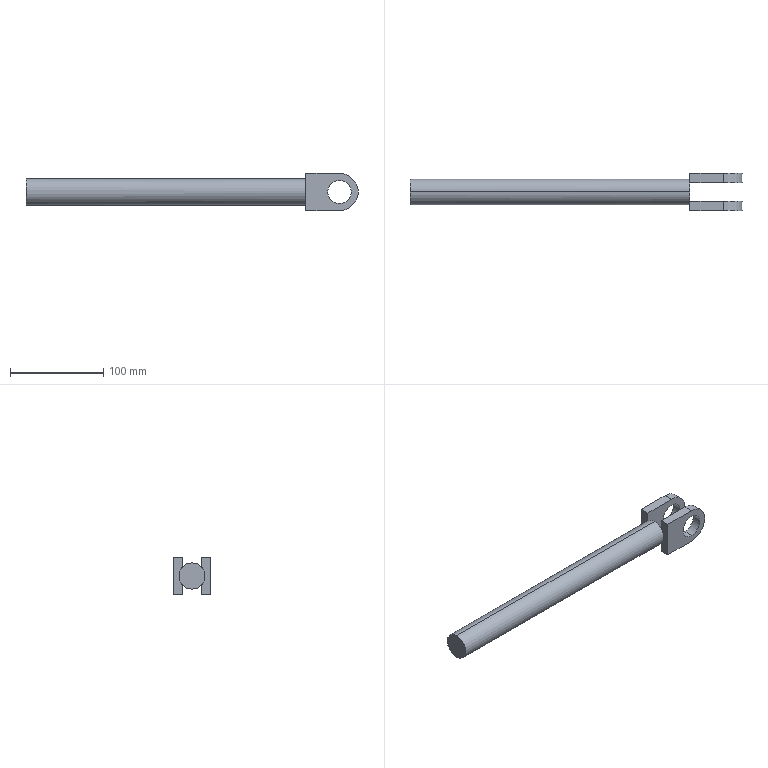Part | SolidWorks | features Extrusion 1, ICE 1, MirrorPattern 1 | 1 solid | 20 faces | box 356.143 x 40 x 40 mm | volume 216389 mm3 | plane 12 | cylinder 8 | commonest cylinder face diameters 25 x4 28 x2 40 x2
STEP:
#1=CARTESIAN_POINT('',(72.286,-30.,-12.5));
#2=VERTEX_POINT('',#1);
#3=CARTESIAN_POINT('',(72.286,-30.,12.5));
#4=VERTEX_POINT('',#3);
#5=CARTESIAN_POINT('',(72.286,-30.,0.));
#6=DIRECTION('',(0.,1.,0.));
#7=DIRECTION('',(0.,0.,1.));
#8=AXIS2_PLACEMENT_3D('',#5,#6,#7);
#9=CIRCLE('',#8,12.5);
#10=EDGE_CURVE('',#2,#4,#9,.T.);
#11=ORIENTED_EDGE('',*,*,#10,.F.);
#12=CARTESIAN_POINT('',(72.286,-20.,-12.5));
#13=VERTEX_POINT('',#12);
#14=CARTESIAN_POINT('',(72.286,-30.,-12.5));
#15=DIRECTION('',(0.,1.,0.));
#16=VECTOR('',#15,1000.);
#17=LINE('',#14,#16);
#18=EDGE_CURVE('',#2,#13,#17,.T.);
#19=ORIENTED_EDGE('',*,*,#18,.T.);
#20=CARTESIAN_POINT('',(72.286,-20.,12.5));
#21=VERTEX_POINT('',#20);
#22=CARTESIAN_POINT('',(72.286,-20.,0.));
#23=DIRECTION('',(0.,1.,0.));
#24=DIRECTION('',(0.,0.,1.));
#25=AXIS2_PLACEMENT_3D('',#22,#23,#24);
#26=CIRCLE('',#25,12.5);
#27=EDGE_CURVE('',#13,#21,#26,.T.);
#28=ORIENTED_EDGE('',*,*,#27,.T.);
#29=CARTESIAN_POINT('',(72.286,-30.,12.5));
#30=DIRECTION('',(0.,1.,0.));
#31=VECTOR('',#30,1000.);
#32=LINE('',#29,#31);
#33=EDGE_CURVE('',#4,#21,#32,.T.);
#34=ORIENTED_EDGE('',*,*,#33,.F.);
#35=EDGE_LOOP('',(#11,#19,#28,#34));
#36=FACE_OUTER_BOUND('',#35,.T.);
#37=CARTESIAN_POINT('',(72.286,-30.,0.));
#38=DIRECTION('',(0.,1.,0.));
#39=DIRECTION('',(0.,0.,1.));
#40=AXIS2_PLACEMENT_3D('',#37,#38,#39);
#41=CYLINDRICAL_SURFACE('',#40,12.5);
#42=ADVANCED_FACE('',(#36),#41,.F.);
#43=CARTESIAN_POINT('',(-263.857,-10.,14.));
#44=VERTEX_POINT('',#43);
#45=CARTESIAN_POINT('',(-263.857,-10.,-14.));
#46=VERTEX_POINT('',#45);
#47=CARTESIAN_POINT('',(-263.857,-10.,0.));
#48=DIRECTION('',(-1.,0.,0.));
#49=DIRECTION('',(0.,0.,1.));
#50=AXIS2_PLACEMENT_3D('',#47,#48,#49);
#51=CIRCLE('',#50,14.);
#52=EDGE_CURVE('',#44,#46,#51,.T.);
#53=ORIENTED_EDGE('',*,*,#52,.F.);
#54=CARTESIAN_POINT('',(36.143,-10.,14.));
#55=VERTEX_POINT('',#54);
#56=CARTESIAN_POINT('',(-263.857,-10.,14.));
#57=DIRECTION('',(1.,0.,0.));
#58=VECTOR('',#57,1000.);
#59=LINE('',#56,#58);
#60=EDGE_CURVE('',#44,#55,#59,.T.);
#61=ORIENTED_EDGE('',*,*,#60,.T.);
#62=CARTESIAN_POINT('',(36.143,0.,9.798));
#63=VERTEX_POINT('',#62);
#64=CARTESIAN_POINT('',(36.143,-10.,0.));
#65=DIRECTION('',(-1.,0.,0.));
#66=DIRECTION('',(0.,0.,1.));
#67=AXIS2_PLACEMENT_3D('',#64,#65,#66);
#68=CIRCLE('',#67,14.);
#69=EDGE_CURVE('',#55,#63,#68,.T.);
#70=ORIENTED_EDGE('',*,*,#69,.T.);
#71=CARTESIAN_POINT('',(36.143,0.,-9.798));
#72=VERTEX_POINT('',#71);
#73=CARTESIAN_POINT('',(36.143,-10.,0.));
#74=DIRECTION('',(-1.,0.,0.));
#75=DIRECTION('',(0.,0.,1.));
#76=AXIS2_PLACEMENT_3D('',#73,#74,#75);
#77=CIRCLE('',#76,14.);
#78=EDGE_CURVE('',#63,#72,#77,.T.);
#79=ORIENTED_EDGE('',*,*,#78,.T.);
#80=CARTESIAN_POINT('',(36.143,-10.,-14.));
#81=VERTEX_POINT('',#80);
#82=CARTESIAN_POINT('',(36.143,-10.,0.));
#83=DIRECTION('',(-1.,0.,0.));
#84=DIRECTION('',(0.,0.,1.));
#85=AXIS2_PLACEMENT_3D('',#82,#83,#84);
#86=CIRCLE('',#85,14.);
#87=EDGE_CURVE('',#72,#81,#86,.T.);
#88=ORIENTED_EDGE('',*,*,#87,.T.);
#89=CARTESIAN_POINT('',(-263.857,-10.,-14.));
#90=DIRECTION('',(1.,0.,0.));
#91=VECTOR('',#90,1000.);
#92=LINE('',#89,#91);
#93=EDGE_CURVE('',#46,#81,#92,.T.);
#94=ORIENTED_EDGE('',*,*,#93,.F.);
#95=EDGE_LOOP('',(#53,#61,#70,#79,#88,#94));
#96=FACE_OUTER_BOUND('',#95,.T.);
#97=CARTESIAN_POINT('',(-263.857,-10.,0.));
#98=DIRECTION('',(1.,0.,0.));
#99=DIRECTION('',(0.,0.,-1.));
#100=AXIS2_PLACEMENT_3D('',#97,#98,#99);
#101=CYLINDRICAL_SURFACE('',#100,14.);
#102=ADVANCED_FACE('',(#96),#101,.T.);
#103=CARTESIAN_POINT('',(72.286,10.,-12.5));
#104=VERTEX_POINT('',#103);
#105=CARTESIAN_POINT('',(72.286,10.,12.5));
#106=VERTEX_POINT('',#105);
#107=CARTESIAN_POINT('',(72.286,10.,0.));
#108=DIRECTION('',(0.,1.,0.));
#109=DIRECTION('',(0.,0.,1.));
#110=AXIS2_PLACEMENT_3D('',#107,#108,#109);
#111=CIRCLE('',#110,12.5);
#112=EDGE_CURVE('',#104,#106,#111,.T.);
#113=ORIENTED_EDGE('',*,*,#112,.T.);
#114=CARTESIAN_POINT('',(72.286,0.,12.5));
#115=VERTEX_POINT('',#114);
#116=CARTESIAN_POINT('',(72.286,10.,12.5));
#117=DIRECTION('',(0.,-1.,0.));
#118=VECTOR('',#117,1000.);
#119=LINE('',#116,#118);
#120=EDGE_CURVE('',#106,#115,#119,.T.);
#121=ORIENTED_EDGE('',*,*,#120,.T.);
#122=CARTESIAN_POINT('',(72.286,0.,-12.5));
#123=VERTEX_POINT('',#122);
#124=CARTESIAN_POINT('',(72.286,0.,0.));
#125=DIRECTION('',(0.,1.,0.));
#126=DIRECTION('',(0.,0.,1.));
#127=AXIS2_PLACEMENT_3D('',#124,#125,#126);
#128=CIRCLE('',#127,12.5);
#129=EDGE_CURVE('',#123,#115,#128,.T.);
#130=ORIENTED_EDGE('',*,*,#129,.F.);
#131=CARTESIAN_POINT('',(72.286,10.,-12.5));
#132=DIRECTION('',(0.,-1.,0.));
#133=VECTOR('',#132,1000.);
#134=LINE('',#131,#133);
#135=EDGE_CURVE('',#104,#123,#134,.T.);
#136=ORIENTED_EDGE('',*,*,#135,.F.);
#137=EDGE_LOOP('',(#113,#121,#130,#136));
#138=FACE_OUTER_BOUND('',#137,.T.);
#139=CARTESIAN_POINT('',(72.286,10.,0.));
#140=DIRECTION('',(0.,-1.,0.));
#141=DIRECTION('',(0.,0.,-1.));
#142=AXIS2_PLACEMENT_3D('',#139,#140,#141);
#143=CYLINDRICAL_SURFACE('',#142,12.5);
#144=ADVANCED_FACE('',(#138),#143,.F.);
#145=CARTESIAN_POINT('',(36.143,-20.,-9.798));
#146=VERTEX_POINT('',#145);
#147=CARTESIAN_POINT('',(36.143,-20.,9.798));
#148=VERTEX_POINT('',#147);
#149=CARTESIAN_POINT('',(36.143,-20.,-20.));
#150=DIRECTION('',(0.,0.,1.));
#151=VECTOR('',#150,1000.);
#152=LINE('',#149,#151);
#153=EDGE_CURVE('',#146,#148,#152,.T.);
#154=ORIENTED_EDGE('',*,*,#153,.F.);
#155=CARTESIAN_POINT('',(36.143,-10.,0.));
#156=DIRECTION('',(-1.,0.,0.));
#157=DIRECTION('',(0.,0.,1.));
#158=AXIS2_PLACEMENT_3D('',#155,#156,#157);
#159=CIRCLE('',#158,14.);
#160=EDGE_CURVE('',#81,#146,#159,.T.);
#161=ORIENTED_EDGE('',*,*,#160,.F.);
#162=ORIENTED_EDGE('',*,*,#87,.F.);
#163=CARTESIAN_POINT('',(36.143,0.,-20.));
#164=DIRECTION('',(0.,0.,1.));
#165=VECTOR('',#164,1000.);
#166=LINE('',#163,#165);
#167=EDGE_CURVE('',#72,#63,#166,.T.);
#168=ORIENTED_EDGE('',*,*,#167,.T.);
#169=ORIENTED_EDGE('',*,*,#69,.F.);
#170=CARTESIAN_POINT('',(36.143,-10.,0.));
#171=DIRECTION('',(-1.,0.,0.));
#172=DIRECTION('',(0.,0.,1.));
#173=AXIS2_PLACEMENT_3D('',#170,#171,#172);
#174=CIRCLE('',#173,14.);
#175=EDGE_CURVE('',#148,#55,#174,.T.);
#176=ORIENTED_EDGE('',*,*,#175,.F.);
#177=EDGE_LOOP('',(#154,#161,#162,#168,#169,#176));
#178=FACE_OUTER_BOUND('',#177,.T.);
#179=CARTESIAN_POINT('',(36.143,-10.,0.));
#180=DIRECTION('',(-1.,0.,0.));
#181=DIRECTION('',(0.,0.,1.));
#182=AXIS2_PLACEMENT_3D('',#179,#180,#181);
#183=PLANE('',#182);
#184=ADVANCED_FACE('',(#178),#183,.F.);
#185=CARTESIAN_POINT('',(72.286,10.,20.));
#186=VERTEX_POINT('',#185);
#187=CARTESIAN_POINT('',(72.286,10.,-20.));
#188=VERTEX_POINT('',#187);
#189=CARTESIAN_POINT('',(72.286,10.,0.));
#190=DIRECTION('',(0.,1.,0.));
#191=DIRECTION('',(0.,0.,1.));
#192=AXIS2_PLACEMENT_3D('',#189,#190,#191);
#193=CIRCLE('',#192,20.);
#194=EDGE_CURVE('',#186,#188,#193,.T.);
#195=ORIENTED_EDGE('',*,*,#194,.T.);
#196=CARTESIAN_POINT('',(36.143,10.,-20.));
#197=VERTEX_POINT('',#196);
#198=CARTESIAN_POINT('',(36.143,10.,-20.));
#199=DIRECTION('',(-1.,0.,0.));
#200=VECTOR('',#199,1000.);
#201=LINE('',#198,#200);
#202=EDGE_CURVE('',#188,#197,#201,.T.);
#203=ORIENTED_EDGE('',*,*,#202,.T.);
#204=CARTESIAN_POINT('',(36.143,10.,20.));
#205=VERTEX_POINT('',#204);
#206=CARTESIAN_POINT('',(36.143,10.,-20.));
#207=DIRECTION('',(0.,0.,1.));
#208=VECTOR('',#207,1000.);
#209=LINE('',#206,#208);
#210=EDGE_CURVE('',#197,#205,#209,.T.);
#211=ORIENTED_EDGE('',*,*,#210,.T.);
#212=CARTESIAN_POINT('',(36.143,10.,20.));
#213=DIRECTION('',(1.,0.,0.));
#214=VECTOR('',#213,1000.);
#215=LINE('',#212,#214);
#216=EDGE_CURVE('',#205,#186,#215,.T.);
#217=ORIENTED_EDGE('',*,*,#216,.T.);
#218=EDGE_LOOP('',(#195,#203,#211,#217));
#219=FACE_OUTER_BOUND('',#218,.T.);
#220=ORIENTED_EDGE('',*,*,#112,.F.);
#221=CARTESIAN_POINT('',(72.286,10.,0.));
#222=DIRECTION('',(0.,1.,0.));
#223=DIRECTION('',(0.,0.,1.));
#224=AXIS2_PLACEMENT_3D('',#221,#222,#223);
#225=CIRCLE('',#224,12.5);
#226=EDGE_CURVE('',#106,#104,#225,.T.);
#227=ORIENTED_EDGE('',*,*,#226,.F.);
#228=EDGE_LOOP('',(#220,#227));
#229=FACE_BOUND('',#228,.T.);
#230=CARTESIAN_POINT('',(72.286,10.,0.));
#231=DIRECTION('',(0.,1.,0.));
#232=DIRECTION('',(0.,0.,1.));
#233=AXIS2_PLACEMENT_3D('',#230,#231,#232);
#234=PLANE('',#233);
#235=ADVANCED_FACE('',(#219,#229),#234,.T.);
#236=CARTESIAN_POINT('',(72.286,0.,20.));
#237=VERTEX_POINT('',#236);
#238=CARTESIAN_POINT('',(72.286,0.,-20.));
#239=VERTEX_POINT('',#238);
#240=CARTESIAN_POINT('',(72.286,0.,0.));
#241=DIRECTION('',(0.,1.,0.));
#242=DIRECTION('',(0.,0.,1.));
#243=AXIS2_PLACEMENT_3D('',#240,#241,#242);
#244=CIRCLE('',#243,20.);
#245=EDGE_CURVE('',#237,#239,#244,.T.);
#246=ORIENTED_EDGE('',*,*,#245,.F.);
#247=CARTESIAN_POINT('',(36.143,0.,20.));
#248=VERTEX_POINT('',#247);
#249=CARTESIAN_POINT('',(36.143,0.,20.));
#250=DIRECTION('',(1.,0.,0.));
#251=VECTOR('',#250,1000.);
#252=LINE('',#249,#251);
#253=EDGE_CURVE('',#248,#237,#252,.T.);
#254=ORIENTED_EDGE('',*,*,#253,.F.);
#255=CARTESIAN_POINT('',(36.143,0.,-20.));
#256=DIRECTION('',(0.,0.,1.));
#257=VECTOR('',#256,1000.);
#258=LINE('',#255,#257);
#259=EDGE_CURVE('',#63,#248,#258,.T.);
#260=ORIENTED_EDGE('',*,*,#259,.F.);
#261=ORIENTED_EDGE('',*,*,#167,.F.);
#262=CARTESIAN_POINT('',(36.143,0.,-20.));
#263=VERTEX_POINT('',#262);
#264=CARTESIAN_POINT('',(36.143,0.,-20.));
#265=DIRECTION('',(0.,0.,1.));
#266=VECTOR('',#265,1000.);
#267=LINE('',#264,#266);
#268=EDGE_CURVE('',#263,#72,#267,.T.);
#269=ORIENTED_EDGE('',*,*,#268,.F.);
#270=CARTESIAN_POINT('',(36.143,0.,-20.));
#271=DIRECTION('',(-1.,0.,0.));
#272=VECTOR('',#271,1000.);
#273=LINE('',#270,#272);
#274=EDGE_CURVE('',#239,#263,#273,.T.);
#275=ORIENTED_EDGE('',*,*,#274,.F.);
#276=EDGE_LOOP('',(#246,#254,#260,#261,#269,#275));
#277=FACE_OUTER_BOUND('',#276,.T.);
#278=ORIENTED_EDGE('',*,*,#129,.T.);
#279=CARTESIAN_POINT('',(72.286,0.,0.));
#280=DIRECTION('',(0.,1.,0.));
#281=DIRECTION('',(0.,0.,1.));
#282=AXIS2_PLACEMENT_3D('',#279,#280,#281);
#283=CIRCLE('',#282,12.5);
#284=EDGE_CURVE('',#115,#123,#283,.T.);
#285=ORIENTED_EDGE('',*,*,#284,.T.);
#286=EDGE_LOOP('',(#278,#285));
#287=FACE_BOUND('',#286,.T.);
#288=CARTESIAN_POINT('',(72.286,0.,0.));
#289=DIRECTION('',(0.,1.,0.));
#290=DIRECTION('',(0.,0.,1.));
#291=AXIS2_PLACEMENT_3D('',#288,#289,#290);
#292=PLANE('',#291);
#293=ADVANCED_FACE('',(#277,#287),#292,.F.);
#294=ORIENTED_EDGE('',*,*,#245,.T.);
#295=CARTESIAN_POINT('',(72.286,10.,-20.));
#296=DIRECTION('',(0.,-1.,0.));
#297=VECTOR('',#296,1000.);
#298=LINE('',#295,#297);
#299=EDGE_CURVE('',#188,#239,#298,.T.);
#300=ORIENTED_EDGE('',*,*,#299,.F.);
#301=ORIENTED_EDGE('',*,*,#194,.F.);
#302=CARTESIAN_POINT('',(72.286,10.,20.));
#303=DIRECTION('',(0.,-1.,0.));
#304=VECTOR('',#303,1000.);
#305=LINE('',#302,#304);
#306=EDGE_CURVE('',#186,#237,#305,.T.);
#307=ORIENTED_EDGE('',*,*,#306,.T.);
#308=EDGE_LOOP('',(#294,#300,#301,#307));
#309=FACE_OUTER_BOUND('',#308,.T.);
#310=CARTESIAN_POINT('',(72.286,10.,0.));
#311=DIRECTION('',(0.,-1.,0.));
#312=DIRECTION('',(0.,0.,-1.));
#313=AXIS2_PLACEMENT_3D('',#310,#311,#312);
#314=CYLINDRICAL_SURFACE('',#313,20.);
#315=ADVANCED_FACE('',(#309),#314,.T.);
#316=ORIENTED_EDGE('',*,*,#274,.T.);
#317=CARTESIAN_POINT('',(36.143,10.,-20.));
#318=DIRECTION('',(0.,-1.,0.));
#319=VECTOR('',#318,1000.);
#320=LINE('',#317,#319);
#321=EDGE_CURVE('',#197,#263,#320,.T.);
#322=ORIENTED_EDGE('',*,*,#321,.F.);
#323=ORIENTED_EDGE('',*,*,#202,.F.);
#324=ORIENTED_EDGE('',*,*,#299,.T.);
#325=EDGE_LOOP('',(#316,#322,#323,#324));
#326=FACE_OUTER_BOUND('',#325,.T.);
#327=CARTESIAN_POINT('',(36.143,10.,-20.));
#328=DIRECTION('',(0.,0.,1.));
#329=DIRECTION('',(1.,0.,0.));
#330=AXIS2_PLACEMENT_3D('',#327,#328,#329);
#331=PLANE('',#330);
#332=ADVANCED_FACE('',(#326),#331,.F.);
#333=ORIENTED_EDGE('',*,*,#78,.F.);
#334=ORIENTED_EDGE('',*,*,#259,.T.);
#335=CARTESIAN_POINT('',(36.143,10.,20.));
#336=DIRECTION('',(0.,-1.,0.));
#337=VECTOR('',#336,1000.);
#338=LINE('',#335,#337);
#339=EDGE_CURVE('',#205,#248,#338,.T.);
#340=ORIENTED_EDGE('',*,*,#339,.F.);
#341=ORIENTED_EDGE('',*,*,#210,.F.);
#342=ORIENTED_EDGE('',*,*,#321,.T.);
#343=ORIENTED_EDGE('',*,*,#268,.T.);
#344=EDGE_LOOP('',(#333,#334,#340,#341,#342,#343));
#345=FACE_OUTER_BOUND('',#344,.T.);
#346=CARTESIAN_POINT('',(36.143,10.,-20.));
#347=DIRECTION('',(1.,0.,0.));
#348=DIRECTION('',(0.,0.,-1.));
#349=AXIS2_PLACEMENT_3D('',#346,#347,#348);
#350=PLANE('',#349);
#351=ADVANCED_FACE('',(#345),#350,.F.);
#352=ORIENTED_EDGE('',*,*,#253,.T.);
#353=ORIENTED_EDGE('',*,*,#306,.F.);
#354=ORIENTED_EDGE('',*,*,#216,.F.);
#355=ORIENTED_EDGE('',*,*,#339,.T.);
#356=EDGE_LOOP('',(#352,#353,#354,#355));
#357=FACE_OUTER_BOUND('',#356,.T.);
#358=CARTESIAN_POINT('',(36.143,10.,20.));
#359=DIRECTION('',(0.,0.,-1.));
#360=DIRECTION('',(-1.,0.,0.));
#361=AXIS2_PLACEMENT_3D('',#358,#359,#360);
#362=PLANE('',#361);
#363=ADVANCED_FACE('',(#357),#362,.F.);
#364=ORIENTED_EDGE('',*,*,#120,.F.);
#365=ORIENTED_EDGE('',*,*,#226,.T.);
#366=ORIENTED_EDGE('',*,*,#135,.T.);
#367=ORIENTED_EDGE('',*,*,#284,.F.);
#368=EDGE_LOOP('',(#364,#365,#366,#367));
#369=FACE_OUTER_BOUND('',#368,.T.);
#370=CARTESIAN_POINT('',(72.286,10.,0.));
#371=DIRECTION('',(0.,-1.,0.));
#372=DIRECTION('',(0.,0.,-1.));
#373=AXIS2_PLACEMENT_3D('',#370,#371,#372);
#374=CYLINDRICAL_SURFACE('',#373,12.5);
#375=ADVANCED_FACE('',(#369),#374,.F.);
#376=ORIENTED_EDGE('',*,*,#60,.F.);
#377=CARTESIAN_POINT('',(-263.857,-10.,0.));
#378=DIRECTION('',(-1.,0.,0.));
#379=DIRECTION('',(0.,0.,1.));
#380=AXIS2_PLACEMENT_3D('',#377,#378,#379);
#381=CIRCLE('',#380,14.);
#382=EDGE_CURVE('',#46,#44,#381,.T.);
#383=ORIENTED_EDGE('',*,*,#382,.F.);
#384=ORIENTED_EDGE('',*,*,#93,.T.);
#385=ORIENTED_EDGE('',*,*,#160,.T.);
#386=CARTESIAN_POINT('',(36.143,-10.,0.));
#387=DIRECTION('',(-1.,0.,0.));
#388=DIRECTION('',(0.,0.,1.));
#389=AXIS2_PLACEMENT_3D('',#386,#387,#388);
#390=CIRCLE('',#389,14.);
#391=EDGE_CURVE('',#146,#148,#390,.T.);
#392=ORIENTED_EDGE('',*,*,#391,.T.);
#393=ORIENTED_EDGE('',*,*,#175,.T.);
#394=EDGE_LOOP('',(#376,#383,#384,#385,#392,#393));
#395=FACE_OUTER_BOUND('',#394,.T.);
#396=CARTESIAN_POINT('',(-263.857,-10.,0.));
#397=DIRECTION('',(1.,0.,0.));
#398=DIRECTION('',(0.,0.,-1.));
#399=AXIS2_PLACEMENT_3D('',#396,#397,#398);
#400=CYLINDRICAL_SURFACE('',#399,14.);
#401=ADVANCED_FACE('',(#395),#400,.T.);
#402=ORIENTED_EDGE('',*,*,#382,.T.);
#403=ORIENTED_EDGE('',*,*,#52,.T.);
#404=EDGE_LOOP('',(#402,#403));
#405=FACE_OUTER_BOUND('',#404,.T.);
#406=CARTESIAN_POINT('',(-263.857,-10.,0.));
#407=DIRECTION('',(-1.,0.,0.));
#408=DIRECTION('',(0.,0.,1.));
#409=AXIS2_PLACEMENT_3D('',#406,#407,#408);
#410=PLANE('',#409);
#411=ADVANCED_FACE('',(#405),#410,.T.);
#412=CARTESIAN_POINT('',(72.286,-20.,20.));
#413=VERTEX_POINT('',#412);
#414=CARTESIAN_POINT('',(72.286,-20.,-20.));
#415=VERTEX_POINT('',#414);
#416=CARTESIAN_POINT('',(72.286,-20.,0.));
#417=DIRECTION('',(0.,1.,0.));
#418=DIRECTION('',(0.,0.,1.));
#419=AXIS2_PLACEMENT_3D('',#416,#417,#418);
#420=CIRCLE('',#419,20.);
#421=EDGE_CURVE('',#413,#415,#420,.T.);
#422=ORIENTED_EDGE('',*,*,#421,.F.);
#423=CARTESIAN_POINT('',(72.286,-30.,20.));
#424=VERTEX_POINT('',#423);
#425=CARTESIAN_POINT('',(72.286,-30.,20.));
#426=DIRECTION('',(0.,1.,0.));
#427=VECTOR('',#426,1000.);
#428=LINE('',#425,#427);
#429=EDGE_CURVE('',#424,#413,#428,.T.);
#430=ORIENTED_EDGE('',*,*,#429,.F.);
#431=CARTESIAN_POINT('',(72.286,-30.,-20.));
#432=VERTEX_POINT('',#431);
#433=CARTESIAN_POINT('',(72.286,-30.,0.));
#434=DIRECTION('',(0.,1.,0.));
#435=DIRECTION('',(0.,0.,1.));
#436=AXIS2_PLACEMENT_3D('',#433,#434,#435);
#437=CIRCLE('',#436,20.);
#438=EDGE_CURVE('',#424,#432,#437,.T.);
#439=ORIENTED_EDGE('',*,*,#438,.T.);
#440=CARTESIAN_POINT('',(72.286,-30.,-20.));
#441=DIRECTION('',(0.,1.,0.));
#442=VECTOR('',#441,1000.);
#443=LINE('',#440,#442);
#444=EDGE_CURVE('',#432,#415,#443,.T.);
#445=ORIENTED_EDGE('',*,*,#444,.T.);
#446=EDGE_LOOP('',(#422,#430,#439,#445));
#447=FACE_OUTER_BOUND('',#446,.T.);
#448=CARTESIAN_POINT('',(72.286,-30.,0.));
#449=DIRECTION('',(0.,1.,0.));
#450=DIRECTION('',(0.,0.,1.));
#451=AXIS2_PLACEMENT_3D('',#448,#449,#450);
#452=CYLINDRICAL_SURFACE('',#451,20.);
#453=ADVANCED_FACE('',(#447),#452,.T.);
#454=CARTESIAN_POINT('',(36.143,-20.,20.));
#455=VERTEX_POINT('',#454);
#456=CARTESIAN_POINT('',(36.143,-20.,20.));
#457=DIRECTION('',(1.,0.,0.));
#458=VECTOR('',#457,1000.);
#459=LINE('',#456,#458);
#460=EDGE_CURVE('',#455,#413,#459,.T.);
#461=ORIENTED_EDGE('',*,*,#460,.F.);
#462=CARTESIAN_POINT('',(36.143,-30.,20.));
#463=VERTEX_POINT('',#462);
#464=CARTESIAN_POINT('',(36.143,-30.,20.));
#465=DIRECTION('',(0.,1.,0.));
#466=VECTOR('',#465,1000.);
#467=LINE('',#464,#466);
#468=EDGE_CURVE('',#463,#455,#467,.T.);
#469=ORIENTED_EDGE('',*,*,#468,.F.);
#470=CARTESIAN_POINT('',(36.143,-30.,20.));
#471=DIRECTION('',(1.,0.,0.));
#472=VECTOR('',#471,1000.);
#473=LINE('',#470,#472);
#474=EDGE_CURVE('',#463,#424,#473,.T.);
#475=ORIENTED_EDGE('',*,*,#474,.T.);
#476=ORIENTED_EDGE('',*,*,#429,.T.);
#477=EDGE_LOOP('',(#461,#469,#475,#476));
#478=FACE_OUTER_BOUND('',#477,.T.);
#479=CARTESIAN_POINT('',(36.143,-30.,20.));
#480=DIRECTION('',(0.,0.,1.));
#481=DIRECTION('',(1.,0.,0.));
#482=AXIS2_PLACEMENT_3D('',#479,#480,#481);
#483=PLANE('',#482);
#484=ADVANCED_FACE('',(#478),#483,.T.);
#485=ORIENTED_EDGE('',*,*,#391,.F.);
#486=CARTESIAN_POINT('',(36.143,-20.,-20.));
#487=VERTEX_POINT('',#486);
#488=CARTESIAN_POINT('',(36.143,-20.,-20.));
#489=DIRECTION('',(0.,0.,1.));
#490=VECTOR('',#489,1000.);
#491=LINE('',#488,#490);
#492=EDGE_CURVE('',#487,#146,#491,.T.);
#493=ORIENTED_EDGE('',*,*,#492,.F.);
#494=CARTESIAN_POINT('',(36.143,-30.,-20.));
#495=VERTEX_POINT('',#494);
#496=CARTESIAN_POINT('',(36.143,-30.,-20.));
#497=DIRECTION('',(0.,1.,0.));
#498=VECTOR('',#497,1000.);
#499=LINE('',#496,#498);
#500=EDGE_CURVE('',#495,#487,#499,.T.);
#501=ORIENTED_EDGE('',*,*,#500,.F.);
#502=CARTESIAN_POINT('',(36.143,-30.,-20.));
#503=DIRECTION('',(0.,0.,1.));
#504=VECTOR('',#503,1000.);
#505=LINE('',#502,#504);
#506=EDGE_CURVE('',#495,#463,#505,.T.);
#507=ORIENTED_EDGE('',*,*,#506,.T.);
#508=ORIENTED_EDGE('',*,*,#468,.T.);
#509=CARTESIAN_POINT('',(36.143,-20.,-20.));
#510=DIRECTION('',(0.,0.,1.));
#511=VECTOR('',#510,1000.);
#512=LINE('',#509,#511);
#513=EDGE_CURVE('',#148,#455,#512,.T.);
#514=ORIENTED_EDGE('',*,*,#513,.F.);
#515=EDGE_LOOP('',(#485,#493,#501,#507,#508,#514));
#516=FACE_OUTER_BOUND('',#515,.T.);
#517=CARTESIAN_POINT('',(36.143,-30.,-20.));
#518=DIRECTION('',(-1.,0.,0.));
#519=DIRECTION('',(0.,0.,1.));
#520=AXIS2_PLACEMENT_3D('',#517,#518,#519);
#521=PLANE('',#520);
#522=ADVANCED_FACE('',(#516),#521,.T.);
#523=CARTESIAN_POINT('',(36.143,-20.,-20.));
#524=DIRECTION('',(-1.,0.,0.));
#525=VECTOR('',#524,1000.);
#526=LINE('',#523,#525);
#527=EDGE_CURVE('',#415,#487,#526,.T.);
#528=ORIENTED_EDGE('',*,*,#527,.F.);
#529=ORIENTED_EDGE('',*,*,#444,.F.);
#530=CARTESIAN_POINT('',(36.143,-30.,-20.));
#531=DIRECTION('',(-1.,0.,0.));
#532=VECTOR('',#531,1000.);
#533=LINE('',#530,#532);
#534=EDGE_CURVE('',#432,#495,#533,.T.);
#535=ORIENTED_EDGE('',*,*,#534,.T.);
#536=ORIENTED_EDGE('',*,*,#500,.T.);
#537=EDGE_LOOP('',(#528,#529,#535,#536));
#538=FACE_OUTER_BOUND('',#537,.T.);
#539=CARTESIAN_POINT('',(36.143,-30.,-20.));
#540=DIRECTION('',(0.,0.,-1.));
#541=DIRECTION('',(-1.,0.,0.));
#542=AXIS2_PLACEMENT_3D('',#539,#540,#541);
#543=PLANE('',#542);
#544=ADVANCED_FACE('',(#538),#543,.T.);
#545=CARTESIAN_POINT('',(72.286,-30.,0.));
#546=DIRECTION('',(0.,1.,0.));
#547=DIRECTION('',(0.,0.,1.));
#548=AXIS2_PLACEMENT_3D('',#545,#546,#547);
#549=CIRCLE('',#548,12.5);
#550=EDGE_CURVE('',#4,#2,#549,.T.);
#551=ORIENTED_EDGE('',*,*,#550,.T.);
#552=ORIENTED_EDGE('',*,*,#10,.T.);
#553=EDGE_LOOP('',(#551,#552));
#554=FACE_BOUND('',#553,.T.);
#555=ORIENTED_EDGE('',*,*,#438,.F.);
#556=ORIENTED_EDGE('',*,*,#474,.F.);
#557=ORIENTED_EDGE('',*,*,#506,.F.);
#558=ORIENTED_EDGE('',*,*,#534,.F.);
#559=EDGE_LOOP('',(#555,#556,#557,#558));
#560=FACE_OUTER_BOUND('',#559,.T.);
#561=CARTESIAN_POINT('',(72.286,-30.,0.));
#562=DIRECTION('',(0.,-1.,0.));
#563=DIRECTION('',(0.,0.,1.));
#564=AXIS2_PLACEMENT_3D('',#561,#562,#563);
#565=PLANE('',#564);
#566=ADVANCED_FACE('',(#554,#560),#565,.T.);
#567=CARTESIAN_POINT('',(72.286,-20.,0.));
#568=DIRECTION('',(0.,1.,0.));
#569=DIRECTION('',(0.,0.,1.));
#570=AXIS2_PLACEMENT_3D('',#567,#568,#569);
#571=CIRCLE('',#570,12.5);
#572=EDGE_CURVE('',#21,#13,#571,.T.);
#573=ORIENTED_EDGE('',*,*,#572,.F.);
#574=ORIENTED_EDGE('',*,*,#27,.F.);
#575=EDGE_LOOP('',(#573,#574));
#576=FACE_BOUND('',#575,.T.);
#577=ORIENTED_EDGE('',*,*,#421,.T.);
#578=ORIENTED_EDGE('',*,*,#527,.T.);
#579=ORIENTED_EDGE('',*,*,#492,.T.);
#580=ORIENTED_EDGE('',*,*,#153,.T.);
#581=ORIENTED_EDGE('',*,*,#513,.T.);
#582=ORIENTED_EDGE('',*,*,#460,.T.);
#583=EDGE_LOOP('',(#577,#578,#579,#580,#581,#582));
#584=FACE_OUTER_BOUND('',#583,.T.);
#585=CARTESIAN_POINT('',(72.286,-20.,0.));
#586=DIRECTION('',(0.,-1.,0.));
#587=DIRECTION('',(0.,0.,1.));
#588=AXIS2_PLACEMENT_3D('',#585,#586,#587);
#589=PLANE('',#588);
#590=ADVANCED_FACE('',(#576,#584),#589,.F.);
#591=ORIENTED_EDGE('',*,*,#18,.F.);
#592=ORIENTED_EDGE('',*,*,#550,.F.);
#593=ORIENTED_EDGE('',*,*,#33,.T.);
#594=ORIENTED_EDGE('',*,*,#572,.T.);
#595=EDGE_LOOP('',(#591,#592,#593,#594));
#596=FACE_OUTER_BOUND('',#595,.T.);
#597=CARTESIAN_POINT('',(72.286,-30.,0.));
#598=DIRECTION('',(0.,1.,0.));
#599=DIRECTION('',(0.,0.,1.));
#600=AXIS2_PLACEMENT_3D('',#597,#598,#599);
#601=CYLINDRICAL_SURFACE('',#600,12.5);
#602=ADVANCED_FACE('',(#596),#601,.F.);
#603=CLOSED_SHELL('',(#42,#102,#144,#184,#235,#293,#315,#332,#351,#363,#375,#401,#411,#453,#484,#522,#544,#566,#590,#602));
#604=MANIFOLD_SOLID_BREP('',#603);
#605=CARTESIAN_POINT('',(0.,0.,0.));
#606=DIRECTION('',(0.,0.,1.));
#607=DIRECTION('',(1.,0.,0.));
#608=AXIS2_PLACEMENT_3D('',#605,#606,#607);
#609=(LENGTH_UNIT()NAMED_UNIT(*)SI_UNIT(.MILLI.,.METRE.));
#610=UNCERTAINTY_MEASURE_WITH_UNIT(LENGTH_MEASURE(0.00001),#609,'','');
#611=(NAMED_UNIT(*)PLANE_ANGLE_UNIT()SI_UNIT($,.RADIAN.));
#612=(NAMED_UNIT(*)SI_UNIT($,.STERADIAN.)SOLID_ANGLE_UNIT());
#613=(GEOMETRIC_REPRESENTATION_CONTEXT(3)GLOBAL_UNCERTAINTY_ASSIGNED_CONTEXT((#610))GLOBAL_UNIT_ASSIGNED_CONTEXT((#609,#611,#612))REPRESENTATION_CONTEXT('',''));
#614=ADVANCED_BREP_SHAPE_REPRESENTATION('',(#604,#608),#613);